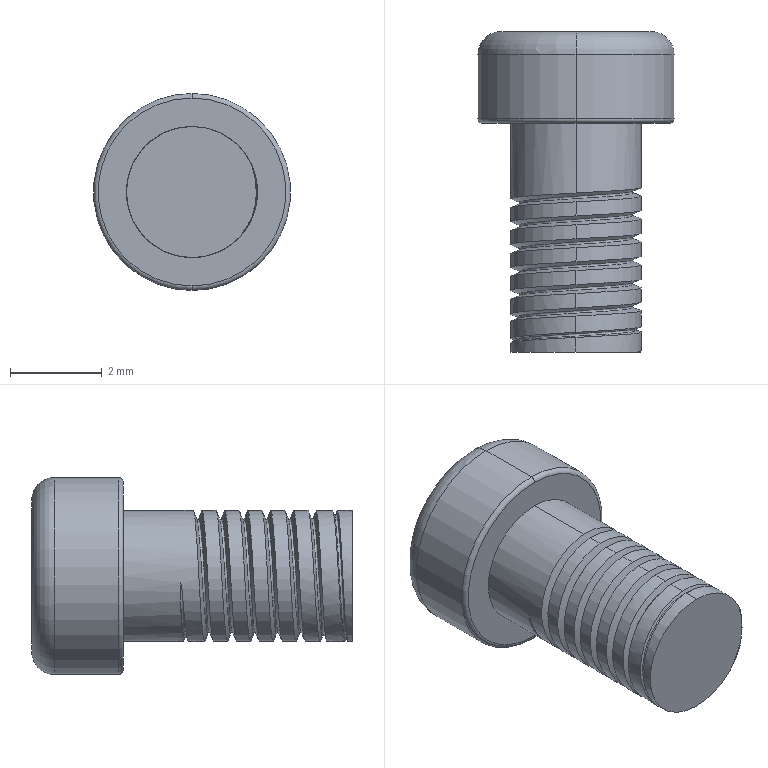Part | SolidWorks | features Helix 3, SweepCut 3, Fillet 2, ICE 2, Extrusion 1 | 1 solid | 49 faces | box 4.3 x 7 x 4.3 mm | volume 56.462 mm3 | cylinder 19 | plane 17 | spline 9 | torus 4 | commonest cylinder face diameters 2.86 x17 4.3 x2